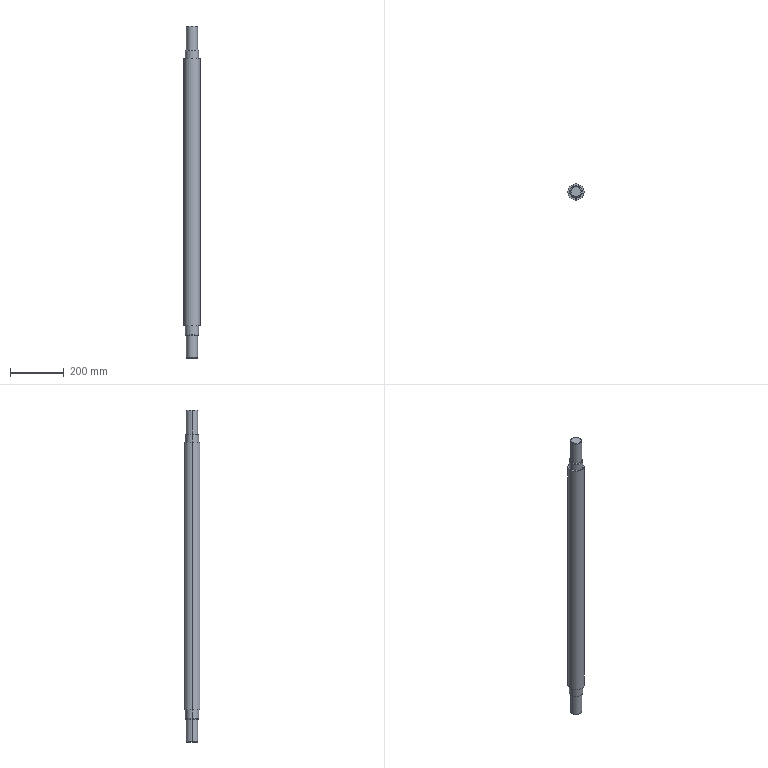Part | SolidWorks | features ICE 4, Chamfer 1, Extrusion 1 | 1 solid | 24 faces | box 60 x 60 x 1240 mm | volume 3194362 mm3 | cylinder 10 | cone 8 | plane 6 | commonest cylinder face diameters 42 x4 49.6 x4 60 x2
STEP:
#1=CARTESIAN_POINT('',(-19.,0.,0.));
#2=VERTEX_POINT('',#1);
#3=CARTESIAN_POINT('',(19.,0.,0.));
#4=VERTEX_POINT('',#3);
#5=CARTESIAN_POINT('',(0.,0.,0.));
#6=DIRECTION('',(0.,0.,-1.));
#7=DIRECTION('',(1.,0.,0.));
#8=AXIS2_PLACEMENT_3D('',#5,#6,#7);
#9=CIRCLE('',#8,19.);
#10=EDGE_CURVE('',#2,#4,#9,.T.);
#11=ORIENTED_EDGE('',*,*,#10,.F.);
#12=CARTESIAN_POINT('',(-21.,0.,2.));
#13=VERTEX_POINT('',#12);
#14=CARTESIAN_POINT('',(-21.,0.,2.));
#15=DIRECTION('',(-0.7071,0.,0.7071));
#16=VECTOR('',#15,1000.);
#17=LINE('',#14,#16);
#18=EDGE_CURVE('',#2,#13,#17,.T.);
#19=ORIENTED_EDGE('',*,*,#18,.T.);
#20=CARTESIAN_POINT('',(21.,0.,2.));
#21=VERTEX_POINT('',#20);
#22=CARTESIAN_POINT('',(0.,0.,2.));
#23=DIRECTION('',(0.,0.,1.));
#24=DIRECTION('',(1.,0.,0.));
#25=AXIS2_PLACEMENT_3D('',#22,#23,#24);
#26=CIRCLE('',#25,21.);
#27=EDGE_CURVE('',#21,#13,#26,.T.);
#28=ORIENTED_EDGE('',*,*,#27,.F.);
#29=CARTESIAN_POINT('',(21.,0.,2.));
#30=DIRECTION('',(0.7071,0.,0.7071));
#31=VECTOR('',#30,1000.);
#32=LINE('',#29,#31);
#33=EDGE_CURVE('',#4,#21,#32,.T.);
#34=ORIENTED_EDGE('',*,*,#33,.F.);
#35=EDGE_LOOP('',(#11,#19,#28,#34));
#36=FACE_OUTER_BOUND('',#35,.T.);
#37=CARTESIAN_POINT('',(0.,0.,2.));
#38=DIRECTION('',(0.,0.,1.));
#39=DIRECTION('',(1.,0.,0.));
#40=AXIS2_PLACEMENT_3D('',#37,#38,#39);
#41=CONICAL_SURFACE('',#40,21.,0.7854);
#42=ADVANCED_FACE('',(#36),#41,.T.);
#43=CARTESIAN_POINT('',(-22.8,0.,85.));
#44=VERTEX_POINT('',#43);
#45=CARTESIAN_POINT('',(22.8,0.,85.));
#46=VERTEX_POINT('',#45);
#47=CARTESIAN_POINT('',(0.,0.,85.));
#48=DIRECTION('',(0.,0.,-1.));
#49=DIRECTION('',(1.,0.,0.));
#50=AXIS2_PLACEMENT_3D('',#47,#48,#49);
#51=CIRCLE('',#50,22.8);
#52=EDGE_CURVE('',#44,#46,#51,.T.);
#53=ORIENTED_EDGE('',*,*,#52,.F.);
#54=CARTESIAN_POINT('',(-24.8,0.,87.));
#55=VERTEX_POINT('',#54);
#56=CARTESIAN_POINT('',(-24.8,0.,87.));
#57=DIRECTION('',(-0.7071,0.,0.7071));
#58=VECTOR('',#57,1000.);
#59=LINE('',#56,#58);
#60=EDGE_CURVE('',#44,#55,#59,.T.);
#61=ORIENTED_EDGE('',*,*,#60,.T.);
#62=CARTESIAN_POINT('',(24.8,0.,87.));
#63=VERTEX_POINT('',#62);
#64=CARTESIAN_POINT('',(0.,0.,87.));
#65=DIRECTION('',(0.,0.,1.));
#66=DIRECTION('',(1.,0.,0.));
#67=AXIS2_PLACEMENT_3D('',#64,#65,#66);
#68=CIRCLE('',#67,24.8);
#69=EDGE_CURVE('',#63,#55,#68,.T.);
#70=ORIENTED_EDGE('',*,*,#69,.F.);
#71=CARTESIAN_POINT('',(24.8,0.,87.));
#72=DIRECTION('',(0.7071,0.,0.7071));
#73=VECTOR('',#72,1000.);
#74=LINE('',#71,#73);
#75=EDGE_CURVE('',#46,#63,#74,.T.);
#76=ORIENTED_EDGE('',*,*,#75,.F.);
#77=EDGE_LOOP('',(#53,#61,#70,#76));
#78=FACE_OUTER_BOUND('',#77,.T.);
#79=CARTESIAN_POINT('',(0.,0.,87.));
#80=DIRECTION('',(0.,0.,1.));
#81=DIRECTION('',(1.,0.,0.));
#82=AXIS2_PLACEMENT_3D('',#79,#80,#81);
#83=CONICAL_SURFACE('',#82,24.8,0.7854);
#84=ADVANCED_FACE('',(#78),#83,.T.);
#85=CARTESIAN_POINT('',(22.8,0.,1150.));
#86=VERTEX_POINT('',#85);
#87=CARTESIAN_POINT('',(-22.8,0.,1150.));
#88=VERTEX_POINT('',#87);
#89=CARTESIAN_POINT('',(0.,0.,1150.));
#90=DIRECTION('',(0.,0.,1.));
#91=DIRECTION('',(1.,0.,0.));
#92=AXIS2_PLACEMENT_3D('',#89,#90,#91);
#93=CIRCLE('',#92,22.8);
#94=EDGE_CURVE('',#86,#88,#93,.T.);
#95=ORIENTED_EDGE('',*,*,#94,.F.);
#96=CARTESIAN_POINT('',(24.8,0.,1148.));
#97=VERTEX_POINT('',#96);
#98=CARTESIAN_POINT('',(22.8,0.,1150.));
#99=DIRECTION('',(0.7071,0.,-0.7071));
#100=VECTOR('',#99,1000.);
#101=LINE('',#98,#100);
#102=EDGE_CURVE('',#86,#97,#101,.T.);
#103=ORIENTED_EDGE('',*,*,#102,.T.);
#104=CARTESIAN_POINT('',(-24.8,0.,1148.));
#105=VERTEX_POINT('',#104);
#106=CARTESIAN_POINT('',(0.,0.,1148.));
#107=DIRECTION('',(0.,0.,-1.));
#108=DIRECTION('',(1.,0.,0.));
#109=AXIS2_PLACEMENT_3D('',#106,#107,#108);
#110=CIRCLE('',#109,24.8);
#111=EDGE_CURVE('',#105,#97,#110,.T.);
#112=ORIENTED_EDGE('',*,*,#111,.F.);
#113=CARTESIAN_POINT('',(-22.8,0.,1150.));
#114=DIRECTION('',(-0.7071,0.,-0.7071));
#115=VECTOR('',#114,1000.);
#116=LINE('',#113,#115);
#117=EDGE_CURVE('',#88,#105,#116,.T.);
#118=ORIENTED_EDGE('',*,*,#117,.F.);
#119=EDGE_LOOP('',(#95,#103,#112,#118));
#120=FACE_OUTER_BOUND('',#119,.T.);
#121=CARTESIAN_POINT('',(0.,0.,1150.));
#122=DIRECTION('',(0.,0.,-1.));
#123=DIRECTION('',(-1.,0.,0.));
#124=AXIS2_PLACEMENT_3D('',#121,#122,#123);
#125=CONICAL_SURFACE('',#124,22.8,0.7854);
#126=ADVANCED_FACE('',(#120),#125,.T.);
#127=CARTESIAN_POINT('',(19.,0.,1240.));
#128=VERTEX_POINT('',#127);
#129=CARTESIAN_POINT('',(-19.,0.,1240.));
#130=VERTEX_POINT('',#129);
#131=CARTESIAN_POINT('',(0.,0.,1240.));
#132=DIRECTION('',(0.,0.,1.));
#133=DIRECTION('',(1.,0.,0.));
#134=AXIS2_PLACEMENT_3D('',#131,#132,#133);
#135=CIRCLE('',#134,19.);
#136=EDGE_CURVE('',#128,#130,#135,.T.);
#137=ORIENTED_EDGE('',*,*,#136,.F.);
#138=CARTESIAN_POINT('',(21.,0.,1238.));
#139=VERTEX_POINT('',#138);
#140=CARTESIAN_POINT('',(19.,0.,1240.));
#141=DIRECTION('',(0.7071,0.,-0.7071));
#142=VECTOR('',#141,1000.);
#143=LINE('',#140,#142);
#144=EDGE_CURVE('',#128,#139,#143,.T.);
#145=ORIENTED_EDGE('',*,*,#144,.T.);
#146=CARTESIAN_POINT('',(-21.,0.,1238.));
#147=VERTEX_POINT('',#146);
#148=CARTESIAN_POINT('',(0.,0.,1238.));
#149=DIRECTION('',(0.,0.,-1.));
#150=DIRECTION('',(1.,0.,0.));
#151=AXIS2_PLACEMENT_3D('',#148,#149,#150);
#152=CIRCLE('',#151,21.);
#153=EDGE_CURVE('',#147,#139,#152,.T.);
#154=ORIENTED_EDGE('',*,*,#153,.F.);
#155=CARTESIAN_POINT('',(-19.,0.,1240.));
#156=DIRECTION('',(-0.7071,0.,-0.7071));
#157=VECTOR('',#156,1000.);
#158=LINE('',#155,#157);
#159=EDGE_CURVE('',#130,#147,#158,.T.);
#160=ORIENTED_EDGE('',*,*,#159,.F.);
#161=EDGE_LOOP('',(#137,#145,#154,#160));
#162=FACE_OUTER_BOUND('',#161,.T.);
#163=CARTESIAN_POINT('',(0.,0.,1240.));
#164=DIRECTION('',(0.,0.,-1.));
#165=DIRECTION('',(-1.,0.,0.));
#166=AXIS2_PLACEMENT_3D('',#163,#164,#165);
#167=CONICAL_SURFACE('',#166,19.,0.7854);
#168=ADVANCED_FACE('',(#162),#167,.T.);
#169=ORIENTED_EDGE('',*,*,#153,.T.);
#170=CARTESIAN_POINT('',(21.,0.,1150.));
#171=VERTEX_POINT('',#170);
#172=CARTESIAN_POINT('',(21.,0.,1240.));
#173=DIRECTION('',(0.,0.,-1.));
#174=VECTOR('',#173,1000.);
#175=LINE('',#172,#174);
#176=EDGE_CURVE('',#139,#171,#175,.T.);
#177=ORIENTED_EDGE('',*,*,#176,.T.);
#178=CARTESIAN_POINT('',(-21.,0.,1150.));
#179=VERTEX_POINT('',#178);
#180=CARTESIAN_POINT('',(0.,0.,1150.));
#181=DIRECTION('',(0.,0.,1.));
#182=DIRECTION('',(1.,0.,0.));
#183=AXIS2_PLACEMENT_3D('',#180,#181,#182);
#184=CIRCLE('',#183,21.);
#185=EDGE_CURVE('',#171,#179,#184,.T.);
#186=ORIENTED_EDGE('',*,*,#185,.T.);
#187=CARTESIAN_POINT('',(-21.,0.,1240.));
#188=DIRECTION('',(0.,0.,-1.));
#189=VECTOR('',#188,1000.);
#190=LINE('',#187,#189);
#191=EDGE_CURVE('',#147,#179,#190,.T.);
#192=ORIENTED_EDGE('',*,*,#191,.F.);
#193=EDGE_LOOP('',(#169,#177,#186,#192));
#194=FACE_OUTER_BOUND('',#193,.T.);
#195=CARTESIAN_POINT('',(0.,0.,1240.));
#196=DIRECTION('',(0.,0.,-1.));
#197=DIRECTION('',(-1.,0.,0.));
#198=AXIS2_PLACEMENT_3D('',#195,#196,#197);
#199=CYLINDRICAL_SURFACE('',#198,21.);
#200=ADVANCED_FACE('',(#194),#199,.T.);
#201=ORIENTED_EDGE('',*,*,#111,.T.);
#202=CARTESIAN_POINT('',(24.8,0.,1120.));
#203=VERTEX_POINT('',#202);
#204=CARTESIAN_POINT('',(24.8,0.,1150.));
#205=DIRECTION('',(0.,0.,-1.));
#206=VECTOR('',#205,1000.);
#207=LINE('',#204,#206);
#208=EDGE_CURVE('',#97,#203,#207,.T.);
#209=ORIENTED_EDGE('',*,*,#208,.T.);
#210=CARTESIAN_POINT('',(-24.8,0.,1120.));
#211=VERTEX_POINT('',#210);
#212=CARTESIAN_POINT('',(0.,0.,1120.));
#213=DIRECTION('',(0.,0.,1.));
#214=DIRECTION('',(1.,0.,0.));
#215=AXIS2_PLACEMENT_3D('',#212,#213,#214);
#216=CIRCLE('',#215,24.8);
#217=EDGE_CURVE('',#203,#211,#216,.T.);
#218=ORIENTED_EDGE('',*,*,#217,.T.);
#219=CARTESIAN_POINT('',(-24.8,0.,1150.));
#220=DIRECTION('',(0.,0.,-1.));
#221=VECTOR('',#220,1000.);
#222=LINE('',#219,#221);
#223=EDGE_CURVE('',#105,#211,#222,.T.);
#224=ORIENTED_EDGE('',*,*,#223,.F.);
#225=EDGE_LOOP('',(#201,#209,#218,#224));
#226=FACE_OUTER_BOUND('',#225,.T.);
#227=CARTESIAN_POINT('',(0.,0.,1150.));
#228=DIRECTION('',(0.,0.,-1.));
#229=DIRECTION('',(-1.,0.,0.));
#230=AXIS2_PLACEMENT_3D('',#227,#228,#229);
#231=CYLINDRICAL_SURFACE('',#230,24.8);
#232=ADVANCED_FACE('',(#226),#231,.T.);
#233=CARTESIAN_POINT('',(30.,0.,1120.));
#234=VERTEX_POINT('',#233);
#235=CARTESIAN_POINT('',(-30.,0.,1120.));
#236=VERTEX_POINT('',#235);
#237=CARTESIAN_POINT('',(0.,0.,1120.));
#238=DIRECTION('',(0.,0.,1.));
#239=DIRECTION('',(1.,0.,0.));
#240=AXIS2_PLACEMENT_3D('',#237,#238,#239);
#241=CIRCLE('',#240,30.);
#242=EDGE_CURVE('',#234,#236,#241,.T.);
#243=ORIENTED_EDGE('',*,*,#242,.F.);
#244=CARTESIAN_POINT('',(30.,0.,120.));
#245=VERTEX_POINT('',#244);
#246=CARTESIAN_POINT('',(30.,0.,1120.));
#247=DIRECTION('',(0.,0.,-1.));
#248=VECTOR('',#247,1000.);
#249=LINE('',#246,#248);
#250=EDGE_CURVE('',#234,#245,#249,.T.);
#251=ORIENTED_EDGE('',*,*,#250,.T.);
#252=CARTESIAN_POINT('',(-30.,0.,120.));
#253=VERTEX_POINT('',#252);
#254=CARTESIAN_POINT('',(0.,0.,120.));
#255=DIRECTION('',(0.,0.,1.));
#256=DIRECTION('',(1.,0.,0.));
#257=AXIS2_PLACEMENT_3D('',#254,#255,#256);
#258=CIRCLE('',#257,30.);
#259=EDGE_CURVE('',#245,#253,#258,.T.);
#260=ORIENTED_EDGE('',*,*,#259,.T.);
#261=CARTESIAN_POINT('',(-30.,0.,1120.));
#262=DIRECTION('',(0.,0.,-1.));
#263=VECTOR('',#262,1000.);
#264=LINE('',#261,#263);
#265=EDGE_CURVE('',#236,#253,#264,.T.);
#266=ORIENTED_EDGE('',*,*,#265,.F.);
#267=EDGE_LOOP('',(#243,#251,#260,#266));
#268=FACE_OUTER_BOUND('',#267,.T.);
#269=CARTESIAN_POINT('',(0.,0.,1120.));
#270=DIRECTION('',(0.,0.,-1.));
#271=DIRECTION('',(-1.,0.,0.));
#272=AXIS2_PLACEMENT_3D('',#269,#270,#271);
#273=CYLINDRICAL_SURFACE('',#272,30.);
#274=ADVANCED_FACE('',(#268),#273,.T.);
#275=CARTESIAN_POINT('',(24.8,0.,120.));
#276=VERTEX_POINT('',#275);
#277=CARTESIAN_POINT('',(-24.8,0.,120.));
#278=VERTEX_POINT('',#277);
#279=CARTESIAN_POINT('',(0.,0.,120.));
#280=DIRECTION('',(0.,0.,1.));
#281=DIRECTION('',(1.,0.,0.));
#282=AXIS2_PLACEMENT_3D('',#279,#280,#281);
#283=CIRCLE('',#282,24.8);
#284=EDGE_CURVE('',#276,#278,#283,.T.);
#285=ORIENTED_EDGE('',*,*,#284,.F.);
#286=CARTESIAN_POINT('',(24.8,0.,120.));
#287=DIRECTION('',(0.,0.,-1.));
#288=VECTOR('',#287,1000.);
#289=LINE('',#286,#288);
#290=EDGE_CURVE('',#276,#63,#289,.T.);
#291=ORIENTED_EDGE('',*,*,#290,.T.);
#292=ORIENTED_EDGE('',*,*,#69,.T.);
#293=CARTESIAN_POINT('',(-24.8,0.,120.));
#294=DIRECTION('',(0.,0.,-1.));
#295=VECTOR('',#294,1000.);
#296=LINE('',#293,#295);
#297=EDGE_CURVE('',#278,#55,#296,.T.);
#298=ORIENTED_EDGE('',*,*,#297,.F.);
#299=EDGE_LOOP('',(#285,#291,#292,#298));
#300=FACE_OUTER_BOUND('',#299,.T.);
#301=CARTESIAN_POINT('',(0.,0.,120.));
#302=DIRECTION('',(0.,0.,-1.));
#303=DIRECTION('',(-1.,0.,0.));
#304=AXIS2_PLACEMENT_3D('',#301,#302,#303);
#305=CYLINDRICAL_SURFACE('',#304,24.8);
#306=ADVANCED_FACE('',(#300),#305,.T.);
#307=CARTESIAN_POINT('',(21.,0.,85.));
#308=VERTEX_POINT('',#307);
#309=CARTESIAN_POINT('',(-21.,0.,85.));
#310=VERTEX_POINT('',#309);
#311=CARTESIAN_POINT('',(0.,0.,85.));
#312=DIRECTION('',(0.,0.,1.));
#313=DIRECTION('',(1.,0.,0.));
#314=AXIS2_PLACEMENT_3D('',#311,#312,#313);
#315=CIRCLE('',#314,21.);
#316=EDGE_CURVE('',#308,#310,#315,.T.);
#317=ORIENTED_EDGE('',*,*,#316,.F.);
#318=CARTESIAN_POINT('',(21.,0.,85.));
#319=DIRECTION('',(0.,0.,-1.));
#320=VECTOR('',#319,1000.);
#321=LINE('',#318,#320);
#322=EDGE_CURVE('',#308,#21,#321,.T.);
#323=ORIENTED_EDGE('',*,*,#322,.T.);
#324=ORIENTED_EDGE('',*,*,#27,.T.);
#325=CARTESIAN_POINT('',(-21.,0.,85.));
#326=DIRECTION('',(0.,0.,-1.));
#327=VECTOR('',#326,1000.);
#328=LINE('',#325,#327);
#329=EDGE_CURVE('',#310,#13,#328,.T.);
#330=ORIENTED_EDGE('',*,*,#329,.F.);
#331=EDGE_LOOP('',(#317,#323,#324,#330));
#332=FACE_OUTER_BOUND('',#331,.T.);
#333=CARTESIAN_POINT('',(0.,0.,85.));
#334=DIRECTION('',(0.,0.,-1.));
#335=DIRECTION('',(-1.,0.,0.));
#336=AXIS2_PLACEMENT_3D('',#333,#334,#335);
#337=CYLINDRICAL_SURFACE('',#336,21.);
#338=ADVANCED_FACE('',(#332),#337,.T.);
#339=ORIENTED_EDGE('',*,*,#322,.F.);
#340=CARTESIAN_POINT('',(0.,0.,85.));
#341=DIRECTION('',(0.,0.,1.));
#342=DIRECTION('',(1.,0.,0.));
#343=AXIS2_PLACEMENT_3D('',#340,#341,#342);
#344=CIRCLE('',#343,21.);
#345=EDGE_CURVE('',#310,#308,#344,.T.);
#346=ORIENTED_EDGE('',*,*,#345,.F.);
#347=ORIENTED_EDGE('',*,*,#329,.T.);
#348=CARTESIAN_POINT('',(0.,0.,2.));
#349=DIRECTION('',(0.,0.,1.));
#350=DIRECTION('',(1.,0.,0.));
#351=AXIS2_PLACEMENT_3D('',#348,#349,#350);
#352=CIRCLE('',#351,21.);
#353=EDGE_CURVE('',#13,#21,#352,.T.);
#354=ORIENTED_EDGE('',*,*,#353,.T.);
#355=EDGE_LOOP('',(#339,#346,#347,#354));
#356=FACE_OUTER_BOUND('',#355,.T.);
#357=CARTESIAN_POINT('',(0.,0.,85.));
#358=DIRECTION('',(0.,0.,-1.));
#359=DIRECTION('',(-1.,0.,0.));
#360=AXIS2_PLACEMENT_3D('',#357,#358,#359);
#361=CYLINDRICAL_SURFACE('',#360,21.);
#362=ADVANCED_FACE('',(#356),#361,.T.);
#363=CARTESIAN_POINT('',(0.,0.,0.));
#364=DIRECTION('',(0.,0.,-1.));
#365=DIRECTION('',(1.,0.,0.));
#366=AXIS2_PLACEMENT_3D('',#363,#364,#365);
#367=CIRCLE('',#366,19.);
#368=EDGE_CURVE('',#4,#2,#367,.T.);
#369=ORIENTED_EDGE('',*,*,#368,.T.);
#370=ORIENTED_EDGE('',*,*,#10,.T.);
#371=EDGE_LOOP('',(#369,#370));
#372=FACE_OUTER_BOUND('',#371,.T.);
#373=CARTESIAN_POINT('',(0.,0.,0.));
#374=DIRECTION('',(0.,0.,1.));
#375=DIRECTION('',(1.,0.,0.));
#376=AXIS2_PLACEMENT_3D('',#373,#374,#375);
#377=PLANE('',#376);
#378=ADVANCED_FACE('',(#372),#377,.F.);
#379=ORIENTED_EDGE('',*,*,#290,.F.);
#380=CARTESIAN_POINT('',(0.,0.,120.));
#381=DIRECTION('',(0.,0.,1.));
#382=DIRECTION('',(1.,0.,0.));
#383=AXIS2_PLACEMENT_3D('',#380,#381,#382);
#384=CIRCLE('',#383,24.8);
#385=EDGE_CURVE('',#278,#276,#384,.T.);
#386=ORIENTED_EDGE('',*,*,#385,.F.);
#387=ORIENTED_EDGE('',*,*,#297,.T.);
#388=CARTESIAN_POINT('',(0.,0.,87.));
#389=DIRECTION('',(0.,0.,1.));
#390=DIRECTION('',(1.,0.,0.));
#391=AXIS2_PLACEMENT_3D('',#388,#389,#390);
#392=CIRCLE('',#391,24.8);
#393=EDGE_CURVE('',#55,#63,#392,.T.);
#394=ORIENTED_EDGE('',*,*,#393,.T.);
#395=EDGE_LOOP('',(#379,#386,#387,#394));
#396=FACE_OUTER_BOUND('',#395,.T.);
#397=CARTESIAN_POINT('',(0.,0.,120.));
#398=DIRECTION('',(0.,0.,-1.));
#399=DIRECTION('',(-1.,0.,0.));
#400=AXIS2_PLACEMENT_3D('',#397,#398,#399);
#401=CYLINDRICAL_SURFACE('',#400,24.8);
#402=ADVANCED_FACE('',(#396),#401,.T.);
#403=CARTESIAN_POINT('',(0.,0.,85.));
#404=DIRECTION('',(0.,0.,-1.));
#405=DIRECTION('',(1.,0.,0.));
#406=AXIS2_PLACEMENT_3D('',#403,#404,#405);
#407=CIRCLE('',#406,22.8);
#408=EDGE_CURVE('',#46,#44,#407,.T.);
#409=ORIENTED_EDGE('',*,*,#408,.T.);
#410=ORIENTED_EDGE('',*,*,#52,.T.);
#411=EDGE_LOOP('',(#409,#410));
#412=FACE_OUTER_BOUND('',#411,.T.);
#413=ORIENTED_EDGE('',*,*,#345,.T.);
#414=ORIENTED_EDGE('',*,*,#316,.T.);
#415=EDGE_LOOP('',(#413,#414));
#416=FACE_BOUND('',#415,.T.);
#417=CARTESIAN_POINT('',(0.,0.,85.));
#418=DIRECTION('',(0.,0.,1.));
#419=DIRECTION('',(1.,0.,0.));
#420=AXIS2_PLACEMENT_3D('',#417,#418,#419);
#421=PLANE('',#420);
#422=ADVANCED_FACE('',(#412,#416),#421,.F.);
#423=ORIENTED_EDGE('',*,*,#250,.F.);
#424=CARTESIAN_POINT('',(0.,0.,1120.));
#425=DIRECTION('',(0.,0.,1.));
#426=DIRECTION('',(1.,0.,0.));
#427=AXIS2_PLACEMENT_3D('',#424,#425,#426);
#428=CIRCLE('',#427,30.);
#429=EDGE_CURVE('',#236,#234,#428,.T.);
#430=ORIENTED_EDGE('',*,*,#429,.F.);
#431=ORIENTED_EDGE('',*,*,#265,.T.);
#432=CARTESIAN_POINT('',(0.,0.,120.));
#433=DIRECTION('',(0.,0.,1.));
#434=DIRECTION('',(1.,0.,0.));
#435=AXIS2_PLACEMENT_3D('',#432,#433,#434);
#436=CIRCLE('',#435,30.);
#437=EDGE_CURVE('',#253,#245,#436,.T.);
#438=ORIENTED_EDGE('',*,*,#437,.T.);
#439=EDGE_LOOP('',(#423,#430,#431,#438));
#440=FACE_OUTER_BOUND('',#439,.T.);
#441=CARTESIAN_POINT('',(0.,0.,1120.));
#442=DIRECTION('',(0.,0.,-1.));
#443=DIRECTION('',(-1.,0.,0.));
#444=AXIS2_PLACEMENT_3D('',#441,#442,#443);
#445=CYLINDRICAL_SURFACE('',#444,30.);
#446=ADVANCED_FACE('',(#440),#445,.T.);
#447=CARTESIAN_POINT('',(0.,0.,1120.));
#448=DIRECTION('',(0.,0.,1.));
#449=DIRECTION('',(1.,0.,0.));
#450=AXIS2_PLACEMENT_3D('',#447,#448,#449);
#451=CIRCLE('',#450,24.8);
#452=EDGE_CURVE('',#211,#203,#451,.T.);
#453=ORIENTED_EDGE('',*,*,#452,.F.);
#454=ORIENTED_EDGE('',*,*,#217,.F.);
#455=EDGE_LOOP('',(#453,#454));
#456=FACE_BOUND('',#455,.T.);
#457=ORIENTED_EDGE('',*,*,#429,.T.);
#458=ORIENTED_EDGE('',*,*,#242,.T.);
#459=EDGE_LOOP('',(#457,#458));
#460=FACE_OUTER_BOUND('',#459,.T.);
#461=CARTESIAN_POINT('',(0.,0.,1120.));
#462=DIRECTION('',(0.,0.,1.));
#463=DIRECTION('',(1.,0.,0.));
#464=AXIS2_PLACEMENT_3D('',#461,#462,#463);
#465=PLANE('',#464);
#466=ADVANCED_FACE('',(#456,#460),#465,.T.);
#467=ORIENTED_EDGE('',*,*,#385,.T.);
#468=ORIENTED_EDGE('',*,*,#284,.T.);
#469=EDGE_LOOP('',(#467,#468));
#470=FACE_BOUND('',#469,.T.);
#471=ORIENTED_EDGE('',*,*,#437,.F.);
#472=ORIENTED_EDGE('',*,*,#259,.F.);
#473=EDGE_LOOP('',(#471,#472));
#474=FACE_OUTER_BOUND('',#473,.T.);
#475=CARTESIAN_POINT('',(0.,0.,120.));
#476=DIRECTION('',(0.,0.,1.));
#477=DIRECTION('',(1.,0.,0.));
#478=AXIS2_PLACEMENT_3D('',#475,#476,#477);
#479=PLANE('',#478);
#480=ADVANCED_FACE('',(#470,#474),#479,.F.);
#481=ORIENTED_EDGE('',*,*,#208,.F.);
#482=CARTESIAN_POINT('',(0.,0.,1148.));
#483=DIRECTION('',(0.,0.,-1.));
#484=DIRECTION('',(1.,0.,0.));
#485=AXIS2_PLACEMENT_3D('',#482,#483,#484);
#486=CIRCLE('',#485,24.8);
#487=EDGE_CURVE('',#97,#105,#486,.T.);
#488=ORIENTED_EDGE('',*,*,#487,.T.);
#489=ORIENTED_EDGE('',*,*,#223,.T.);
#490=ORIENTED_EDGE('',*,*,#452,.T.);
#491=EDGE_LOOP('',(#481,#488,#489,#490));
#492=FACE_OUTER_BOUND('',#491,.T.);
#493=CARTESIAN_POINT('',(0.,0.,1150.));
#494=DIRECTION('',(0.,0.,-1.));
#495=DIRECTION('',(-1.,0.,0.));
#496=AXIS2_PLACEMENT_3D('',#493,#494,#495);
#497=CYLINDRICAL_SURFACE('',#496,24.8);
#498=ADVANCED_FACE('',(#492),#497,.T.);
#499=CARTESIAN_POINT('',(0.,0.,1150.));
#500=DIRECTION('',(0.,0.,1.));
#501=DIRECTION('',(1.,0.,0.));
#502=AXIS2_PLACEMENT_3D('',#499,#500,#501);
#503=CIRCLE('',#502,22.8);
#504=EDGE_CURVE('',#88,#86,#503,.T.);
#505=ORIENTED_EDGE('',*,*,#504,.T.);
#506=ORIENTED_EDGE('',*,*,#94,.T.);
#507=EDGE_LOOP('',(#505,#506));
#508=FACE_OUTER_BOUND('',#507,.T.);
#509=CARTESIAN_POINT('',(0.,0.,1150.));
#510=DIRECTION('',(0.,0.,1.));
#511=DIRECTION('',(1.,0.,0.));
#512=AXIS2_PLACEMENT_3D('',#509,#510,#511);
#513=CIRCLE('',#512,21.);
#514=EDGE_CURVE('',#179,#171,#513,.T.);
#515=ORIENTED_EDGE('',*,*,#514,.F.);
#516=ORIENTED_EDGE('',*,*,#185,.F.);
#517=EDGE_LOOP('',(#515,#516));
#518=FACE_BOUND('',#517,.T.);
#519=CARTESIAN_POINT('',(0.,0.,1150.));
#520=DIRECTION('',(0.,0.,1.));
#521=DIRECTION('',(1.,0.,0.));
#522=AXIS2_PLACEMENT_3D('',#519,#520,#521);
#523=PLANE('',#522);
#524=ADVANCED_FACE('',(#508,#518),#523,.T.);
#525=ORIENTED_EDGE('',*,*,#176,.F.);
#526=CARTESIAN_POINT('',(0.,0.,1238.));
#527=DIRECTION('',(0.,0.,-1.));
#528=DIRECTION('',(1.,0.,0.));
#529=AXIS2_PLACEMENT_3D('',#526,#527,#528);
#530=CIRCLE('',#529,21.);
#531=EDGE_CURVE('',#139,#147,#530,.T.);
#532=ORIENTED_EDGE('',*,*,#531,.T.);
#533=ORIENTED_EDGE('',*,*,#191,.T.);
#534=ORIENTED_EDGE('',*,*,#514,.T.);
#535=EDGE_LOOP('',(#525,#532,#533,#534));
#536=FACE_OUTER_BOUND('',#535,.T.);
#537=CARTESIAN_POINT('',(0.,0.,1240.));
#538=DIRECTION('',(0.,0.,-1.));
#539=DIRECTION('',(-1.,0.,0.));
#540=AXIS2_PLACEMENT_3D('',#537,#538,#539);
#541=CYLINDRICAL_SURFACE('',#540,21.);
#542=ADVANCED_FACE('',(#536),#541,.T.);
#543=CARTESIAN_POINT('',(0.,0.,1240.));
#544=DIRECTION('',(0.,0.,1.));
#545=DIRECTION('',(1.,0.,0.));
#546=AXIS2_PLACEMENT_3D('',#543,#544,#545);
#547=CIRCLE('',#546,19.);
#548=EDGE_CURVE('',#130,#128,#547,.T.);
#549=ORIENTED_EDGE('',*,*,#548,.T.);
#550=ORIENTED_EDGE('',*,*,#136,.T.);
#551=EDGE_LOOP('',(#549,#550));
#552=FACE_OUTER_BOUND('',#551,.T.);
#553=CARTESIAN_POINT('',(0.,0.,1240.));
#554=DIRECTION('',(0.,0.,1.));
#555=DIRECTION('',(1.,0.,0.));
#556=AXIS2_PLACEMENT_3D('',#553,#554,#555);
#557=PLANE('',#556);
#558=ADVANCED_FACE('',(#552),#557,.T.);
#559=ORIENTED_EDGE('',*,*,#144,.F.);
#560=ORIENTED_EDGE('',*,*,#548,.F.);
#561=ORIENTED_EDGE('',*,*,#159,.T.);
#562=ORIENTED_EDGE('',*,*,#531,.F.);
#563=EDGE_LOOP('',(#559,#560,#561,#562));
#564=FACE_OUTER_BOUND('',#563,.T.);
#565=CARTESIAN_POINT('',(0.,0.,1240.));
#566=DIRECTION('',(0.,0.,-1.));
#567=DIRECTION('',(-1.,0.,0.));
#568=AXIS2_PLACEMENT_3D('',#565,#566,#567);
#569=CONICAL_SURFACE('',#568,19.,0.7854);
#570=ADVANCED_FACE('',(#564),#569,.T.);
#571=ORIENTED_EDGE('',*,*,#102,.F.);
#572=ORIENTED_EDGE('',*,*,#504,.F.);
#573=ORIENTED_EDGE('',*,*,#117,.T.);
#574=ORIENTED_EDGE('',*,*,#487,.F.);
#575=EDGE_LOOP('',(#571,#572,#573,#574));
#576=FACE_OUTER_BOUND('',#575,.T.);
#577=CARTESIAN_POINT('',(0.,0.,1150.));
#578=DIRECTION('',(0.,0.,-1.));
#579=DIRECTION('',(-1.,0.,0.));
#580=AXIS2_PLACEMENT_3D('',#577,#578,#579);
#581=CONICAL_SURFACE('',#580,22.8,0.7854);
#582=ADVANCED_FACE('',(#576),#581,.T.);
#583=ORIENTED_EDGE('',*,*,#60,.F.);
#584=ORIENTED_EDGE('',*,*,#408,.F.);
#585=ORIENTED_EDGE('',*,*,#75,.T.);
#586=ORIENTED_EDGE('',*,*,#393,.F.);
#587=EDGE_LOOP('',(#583,#584,#585,#586));
#588=FACE_OUTER_BOUND('',#587,.T.);
#589=CARTESIAN_POINT('',(0.,0.,87.));
#590=DIRECTION('',(0.,0.,1.));
#591=DIRECTION('',(1.,0.,0.));
#592=AXIS2_PLACEMENT_3D('',#589,#590,#591);
#593=CONICAL_SURFACE('',#592,24.8,0.7854);
#594=ADVANCED_FACE('',(#588),#593,.T.);
#595=ORIENTED_EDGE('',*,*,#18,.F.);
#596=ORIENTED_EDGE('',*,*,#368,.F.);
#597=ORIENTED_EDGE('',*,*,#33,.T.);
#598=ORIENTED_EDGE('',*,*,#353,.F.);
#599=EDGE_LOOP('',(#595,#596,#597,#598));
#600=FACE_OUTER_BOUND('',#599,.T.);
#601=CARTESIAN_POINT('',(0.,0.,2.));
#602=DIRECTION('',(0.,0.,1.));
#603=DIRECTION('',(1.,0.,0.));
#604=AXIS2_PLACEMENT_3D('',#601,#602,#603);
#605=CONICAL_SURFACE('',#604,21.,0.7854);
#606=ADVANCED_FACE('',(#600),#605,.T.);
#607=CLOSED_SHELL('',(#42,#84,#126,#168,#200,#232,#274,#306,#338,#362,#378,#402,#422,#446,#466,#480,#498,#524,#542,#558,#570,#582,#594,#606));
#608=MANIFOLD_SOLID_BREP('',#607);
#609=CARTESIAN_POINT('',(0.,0.,0.));
#610=DIRECTION('',(0.,0.,1.));
#611=DIRECTION('',(1.,0.,0.));
#612=AXIS2_PLACEMENT_3D('',#609,#610,#611);
#613=(LENGTH_UNIT()NAMED_UNIT(*)SI_UNIT(.MILLI.,.METRE.));
#614=UNCERTAINTY_MEASURE_WITH_UNIT(LENGTH_MEASURE(0.00001),#613,'','');
#615=(NAMED_UNIT(*)PLANE_ANGLE_UNIT()SI_UNIT($,.RADIAN.));
#616=(NAMED_UNIT(*)SI_UNIT($,.STERADIAN.)SOLID_ANGLE_UNIT());
#617=(GEOMETRIC_REPRESENTATION_CONTEXT(3)GLOBAL_UNCERTAINTY_ASSIGNED_CONTEXT((#614))GLOBAL_UNIT_ASSIGNED_CONTEXT((#613,#615,#616))REPRESENTATION_CONTEXT('',''));
#618=ADVANCED_BREP_SHAPE_REPRESENTATION('',(#608,#612),#617);